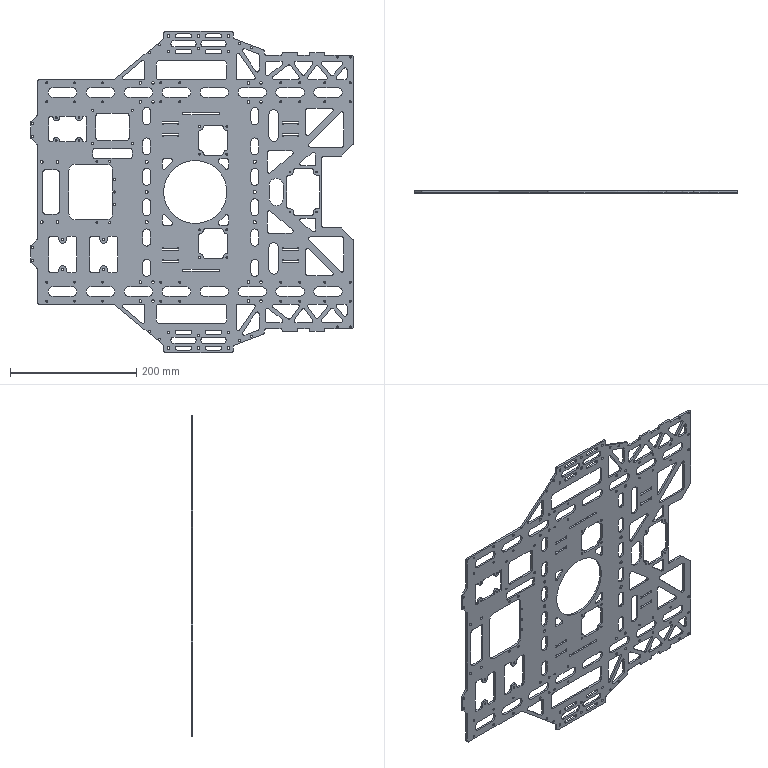Part | SolidWorks | features ICE 16, Fillet 6, Chamfer 2, Extrusion 1 | 1 solid | 1017 faces | box 510.5 x 3 x 508 mm | volume 398593 mm3 | cylinder 703 | plane 314 | commonest cylinder face diameters 6 x232 3.2 x150 4.2 x64 1.5 x60 12 x50 15 x38